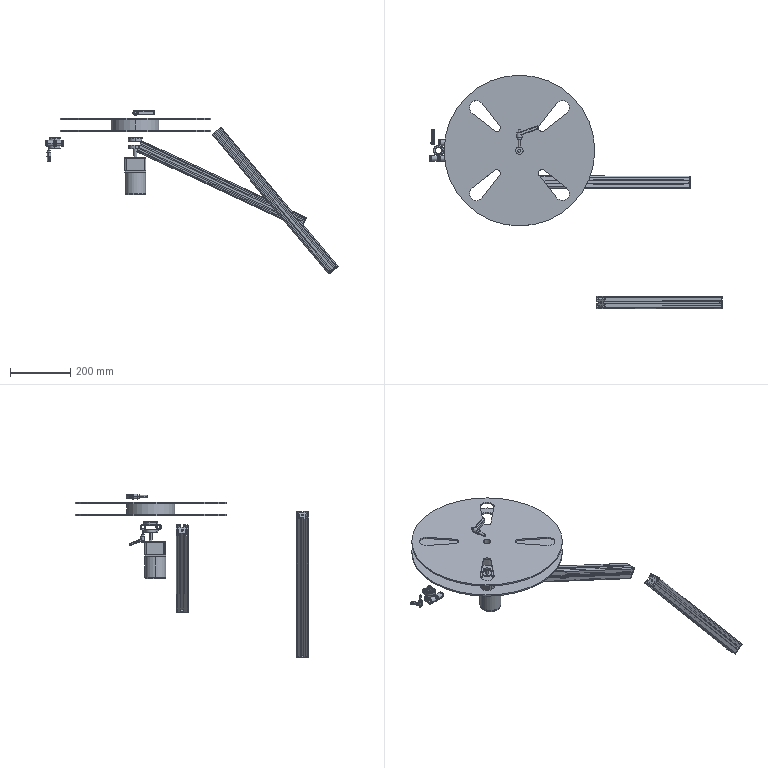Part | NX | 15 solids | 675 faces | box 969.637 x 774 x 544.103 mm | volume 4156414 mm3 | cylinder 260 | plane 258 | cone 68 | torus 57 | spline 22 | sphere 10 | commonest cylinder face diameters 8 x34 10 x18 19 x18 25 x18 1 x16 5.5 x16